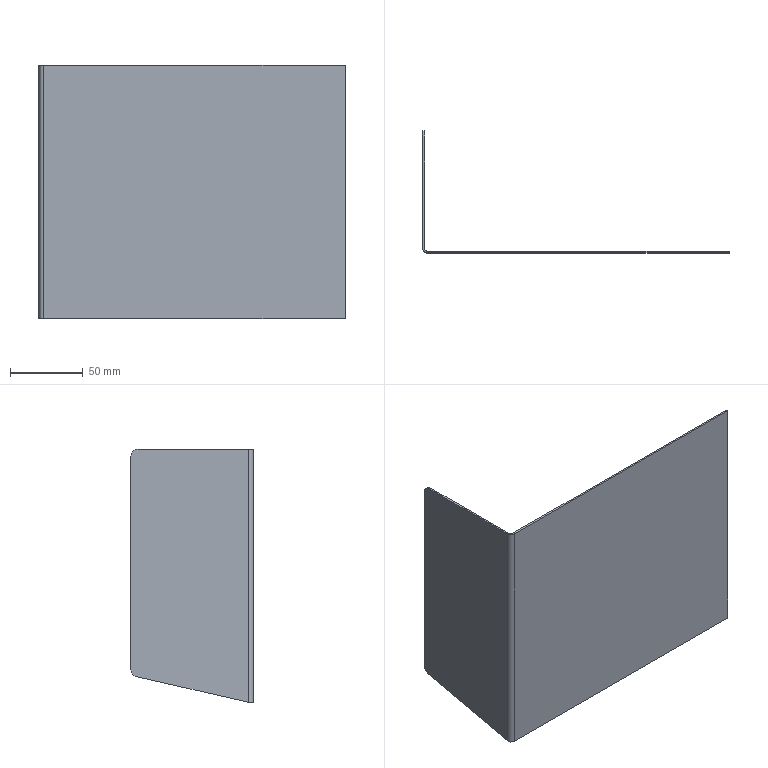Part | SolidWorks | features Fillet 1, FlatPattern 1, ICE 1, SMBaseFlange 1, SheetMetal 1 | 1 solid | 17 faces | box 211.2 x 84.2 x 175 mm | volume 60591 mm3 | plane 12 | cylinder 4 | spline 1 | commonest cylinder face diameters 10 x2 4 x1 6.4 x1
STEP:
#1=CARTESIAN_POINT('',(0.702,-83.,0.));
#2=VERTEX_POINT('',#1);
#3=CARTESIAN_POINT('',(3.2,-84.2,0.));
#4=VERTEX_POINT('',#3);
#5=CARTESIAN_POINT('',(3.2,-81.,0.));
#6=DIRECTION('',(0.,0.,1.));
#7=DIRECTION('',(-1.,0.,0.));
#8=AXIS2_PLACEMENT_3D('',#5,#6,#7);
#9=CIRCLE('',#8,3.2);
#10=EDGE_CURVE('',#2,#4,#9,.T.);
#11=ORIENTED_EDGE('',*,*,#10,.F.);
#12=CARTESIAN_POINT('',(1.639,-82.25,0.));
#13=VERTEX_POINT('',#12);
#14=CARTESIAN_POINT('',(0.702,-83.,0.));
#15=DIRECTION('',(0.7806,0.625,0.));
#16=VECTOR('',#15,1000.);
#17=LINE('',#14,#16);
#18=EDGE_CURVE('',#2,#13,#17,.T.);
#19=ORIENTED_EDGE('',*,*,#18,.T.);
#20=CARTESIAN_POINT('',(3.2,-83.,0.));
#21=VERTEX_POINT('',#20);
#22=CARTESIAN_POINT('',(3.2,-81.,0.));
#23=DIRECTION('',(0.,0.,1.));
#24=DIRECTION('',(1.,0.,0.));
#25=AXIS2_PLACEMENT_3D('',#22,#23,#24);
#26=CIRCLE('',#25,2.);
#27=EDGE_CURVE('',#13,#21,#26,.T.);
#28=ORIENTED_EDGE('',*,*,#27,.T.);
#29=CARTESIAN_POINT('',(3.2,-84.2,0.));
#30=DIRECTION('',(0.,1.,0.));
#31=VECTOR('',#30,1000.);
#32=LINE('',#29,#31);
#33=EDGE_CURVE('',#4,#21,#32,.T.);
#34=ORIENTED_EDGE('',*,*,#33,.F.);
#35=EDGE_LOOP('',(#11,#19,#28,#34));
#36=FACE_OUTER_BOUND('',#35,.T.);
#37=CARTESIAN_POINT('',(3.2,-84.2,0.));
#38=DIRECTION('',(0.,0.,-1.));
#39=DIRECTION('',(-1.,0.,0.));
#40=AXIS2_PLACEMENT_3D('',#37,#38,#39);
#41=PLANE('',#40);
#42=ADVANCED_FACE('',(#36),#41,.T.);
#43=ORIENTED_EDGE('',*,*,#27,.F.);
#44=CARTESIAN_POINT('',(1.2,-81.,0.4578));
#45=VERTEX_POINT('',#44);
#46=CARTESIAN_POINT('',(1.639,-82.25,0.));
#47=CARTESIAN_POINT('',(1.352,-81.892,0.1312));
#48=CARTESIAN_POINT('',(1.2,-81.459,0.2898));
#49=CARTESIAN_POINT('',(1.2,-81.,0.4578));
#50=(BOUNDED_CURVE()B_SPLINE_CURVE(3,(#46,#47,#48,#49),.UNSPECIFIED.,.F.,.T.)B_SPLINE_CURVE_WITH_KNOTS((4,4),(0.8957,1.571),.UNSPECIFIED.)CURVE()GEOMETRIC_REPRESENTATION_ITEM()RATIONAL_B_SPLINE_CURVE((1.,0.9624,0.9624,1.))REPRESENTATION_ITEM(''));
#51=EDGE_CURVE('',#13,#45,#50,.T.);
#52=ORIENTED_EDGE('',*,*,#51,.T.);
#53=CARTESIAN_POINT('',(1.2,-81.,175.));
#54=VERTEX_POINT('',#53);
#55=CARTESIAN_POINT('',(1.2,-81.,175.));
#56=DIRECTION('',(0.,0.,-1.));
#57=VECTOR('',#56,1000.);
#58=LINE('',#55,#57);
#59=EDGE_CURVE('',#54,#45,#58,.T.);
#60=ORIENTED_EDGE('',*,*,#59,.F.);
#61=CARTESIAN_POINT('',(3.2,-83.,175.));
#62=VERTEX_POINT('',#61);
#63=CARTESIAN_POINT('',(3.2,-81.,175.));
#64=DIRECTION('',(0.,0.,1.));
#65=DIRECTION('',(1.,0.,0.));
#66=AXIS2_PLACEMENT_3D('',#63,#64,#65);
#67=CIRCLE('',#66,2.);
#68=EDGE_CURVE('',#54,#62,#67,.T.);
#69=ORIENTED_EDGE('',*,*,#68,.T.);
#70=CARTESIAN_POINT('',(3.2,-83.,175.));
#71=DIRECTION('',(0.,0.,-1.));
#72=VECTOR('',#71,1000.);
#73=LINE('',#70,#72);
#74=EDGE_CURVE('',#62,#21,#73,.T.);
#75=ORIENTED_EDGE('',*,*,#74,.T.);
#76=EDGE_LOOP('',(#43,#52,#60,#69,#75));
#77=FACE_OUTER_BOUND('',#76,.T.);
#78=CARTESIAN_POINT('',(3.2,-81.,175.));
#79=DIRECTION('',(0.,0.,-1.));
#80=DIRECTION('',(-1.,0.,0.));
#81=AXIS2_PLACEMENT_3D('',#78,#79,#80);
#82=CYLINDRICAL_SURFACE('',#81,2.);
#83=ADVANCED_FACE('',(#77),#82,.F.);
#84=CARTESIAN_POINT('',(1.2,-3.884,18.111));
#85=VERTEX_POINT('',#84);
#86=CARTESIAN_POINT('',(1.2,0.,19.));
#87=DIRECTION('',(0.,0.9748,0.2231));
#88=VECTOR('',#87,1000.);
#89=LINE('',#86,#88);
#90=EDGE_CURVE('',#45,#85,#89,.T.);
#91=ORIENTED_EDGE('',*,*,#90,.T.);
#92=CARTESIAN_POINT('',(1.2,0.,22.985));
#93=VERTEX_POINT('',#92);
#94=CARTESIAN_POINT('',(1.2,-5.,22.985));
#95=DIRECTION('',(1.,0.,0.));
#96=DIRECTION('',(0.,1.,0.));
#97=AXIS2_PLACEMENT_3D('',#94,#95,#96);
#98=CIRCLE('',#97,5.);
#99=EDGE_CURVE('',#85,#93,#98,.T.);
#100=ORIENTED_EDGE('',*,*,#99,.T.);
#101=CARTESIAN_POINT('',(1.2,0.,170.));
#102=VERTEX_POINT('',#101);
#103=CARTESIAN_POINT('',(1.2,0.,175.));
#104=DIRECTION('',(0.,0.,-1.));
#105=VECTOR('',#104,1000.);
#106=LINE('',#103,#105);
#107=EDGE_CURVE('',#102,#93,#106,.T.);
#108=ORIENTED_EDGE('',*,*,#107,.F.);
#109=CARTESIAN_POINT('',(1.2,-5.,175.));
#110=VERTEX_POINT('',#109);
#111=CARTESIAN_POINT('',(1.2,-5.,170.));
#112=DIRECTION('',(1.,0.,0.));
#113=DIRECTION('',(0.,1.,0.));
#114=AXIS2_PLACEMENT_3D('',#111,#112,#113);
#115=CIRCLE('',#114,5.);
#116=EDGE_CURVE('',#102,#110,#115,.T.);
#117=ORIENTED_EDGE('',*,*,#116,.T.);
#118=CARTESIAN_POINT('',(1.2,0.,175.));
#119=DIRECTION('',(0.,-1.,0.));
#120=VECTOR('',#119,1000.);
#121=LINE('',#118,#120);
#122=EDGE_CURVE('',#110,#54,#121,.T.);
#123=ORIENTED_EDGE('',*,*,#122,.T.);
#124=ORIENTED_EDGE('',*,*,#59,.T.);
#125=EDGE_LOOP('',(#91,#100,#108,#117,#123,#124));
#126=FACE_OUTER_BOUND('',#125,.T.);
#127=CARTESIAN_POINT('',(1.2,0.,175.));
#128=DIRECTION('',(1.,0.,0.));
#129=DIRECTION('',(0.,1.,0.));
#130=AXIS2_PLACEMENT_3D('',#127,#128,#129);
#131=PLANE('',#130);
#132=ADVANCED_FACE('',(#126),#131,.T.);
#133=ORIENTED_EDGE('',*,*,#107,.T.);
#134=CARTESIAN_POINT('',(0.,0.,22.985));
#135=VERTEX_POINT('',#134);
#136=CARTESIAN_POINT('',(0.,0.,22.985));
#137=DIRECTION('',(-1.,0.,0.));
#138=VECTOR('',#137,1000.);
#139=LINE('',#136,#138);
#140=EDGE_CURVE('',#93,#135,#139,.T.);
#141=ORIENTED_EDGE('',*,*,#140,.T.);
#142=CARTESIAN_POINT('',(0.,0.,170.));
#143=VERTEX_POINT('',#142);
#144=CARTESIAN_POINT('',(0.,0.,175.));
#145=DIRECTION('',(0.,0.,-1.));
#146=VECTOR('',#145,1000.);
#147=LINE('',#144,#146);
#148=EDGE_CURVE('',#143,#135,#147,.T.);
#149=ORIENTED_EDGE('',*,*,#148,.F.);
#150=CARTESIAN_POINT('',(0.,0.,170.));
#151=DIRECTION('',(1.,0.,0.));
#152=VECTOR('',#151,1000.);
#153=LINE('',#150,#152);
#154=EDGE_CURVE('',#143,#102,#153,.T.);
#155=ORIENTED_EDGE('',*,*,#154,.T.);
#156=EDGE_LOOP('',(#133,#141,#149,#155));
#157=FACE_OUTER_BOUND('',#156,.T.);
#158=CARTESIAN_POINT('',(0.,0.,175.));
#159=DIRECTION('',(0.,1.,0.));
#160=DIRECTION('',(-1.,0.,0.));
#161=AXIS2_PLACEMENT_3D('',#158,#159,#160);
#162=PLANE('',#161);
#163=ADVANCED_FACE('',(#157),#162,.T.);
#164=ORIENTED_EDGE('',*,*,#148,.T.);
#165=CARTESIAN_POINT('',(0.,-3.884,18.111));
#166=VERTEX_POINT('',#165);
#167=CARTESIAN_POINT('',(0.,-5.,22.985));
#168=DIRECTION('',(-1.,0.,0.));
#169=DIRECTION('',(0.,1.,0.));
#170=AXIS2_PLACEMENT_3D('',#167,#168,#169);
#171=CIRCLE('',#170,5.);
#172=EDGE_CURVE('',#135,#166,#171,.T.);
#173=ORIENTED_EDGE('',*,*,#172,.T.);
#174=CARTESIAN_POINT('',(0.,-81.,0.4578));
#175=VERTEX_POINT('',#174);
#176=CARTESIAN_POINT('',(0.,0.,19.));
#177=DIRECTION('',(0.,0.9748,0.2231));
#178=VECTOR('',#177,1000.);
#179=LINE('',#176,#178);
#180=EDGE_CURVE('',#175,#166,#179,.T.);
#181=ORIENTED_EDGE('',*,*,#180,.F.);
#182=CARTESIAN_POINT('',(0.,-81.,175.));
#183=VERTEX_POINT('',#182);
#184=CARTESIAN_POINT('',(0.,-81.,175.));
#185=DIRECTION('',(0.,0.,-1.));
#186=VECTOR('',#185,1000.);
#187=LINE('',#184,#186);
#188=EDGE_CURVE('',#183,#175,#187,.T.);
#189=ORIENTED_EDGE('',*,*,#188,.F.);
#190=CARTESIAN_POINT('',(0.,-5.,175.));
#191=VERTEX_POINT('',#190);
#192=CARTESIAN_POINT('',(0.,0.,175.));
#193=DIRECTION('',(0.,-1.,0.));
#194=VECTOR('',#193,1000.);
#195=LINE('',#192,#194);
#196=EDGE_CURVE('',#191,#183,#195,.T.);
#197=ORIENTED_EDGE('',*,*,#196,.F.);
#198=CARTESIAN_POINT('',(0.,-5.,170.));
#199=DIRECTION('',(-1.,0.,0.));
#200=DIRECTION('',(0.,1.,0.));
#201=AXIS2_PLACEMENT_3D('',#198,#199,#200);
#202=CIRCLE('',#201,5.);
#203=EDGE_CURVE('',#191,#143,#202,.T.);
#204=ORIENTED_EDGE('',*,*,#203,.T.);
#205=EDGE_LOOP('',(#164,#173,#181,#189,#197,#204));
#206=FACE_OUTER_BOUND('',#205,.T.);
#207=CARTESIAN_POINT('',(0.,0.,175.));
#208=DIRECTION('',(1.,0.,0.));
#209=DIRECTION('',(0.,1.,0.));
#210=AXIS2_PLACEMENT_3D('',#207,#208,#209);
#211=PLANE('',#210);
#212=ADVANCED_FACE('',(#206),#211,.F.);
#213=CARTESIAN_POINT('',(0.702,-83.,0.));
#214=CARTESIAN_POINT('',(0.2431,-82.427,0.1312));
#215=CARTESIAN_POINT('',(0.,-81.734,0.2898));
#216=CARTESIAN_POINT('',(0.,-81.,0.4578));
#217=(BOUNDED_CURVE()B_SPLINE_CURVE(3,(#213,#214,#215,#216),.UNSPECIFIED.,.F.,.T.)B_SPLINE_CURVE_WITH_KNOTS((4,4),(0.8957,1.571),.UNSPECIFIED.)CURVE()GEOMETRIC_REPRESENTATION_ITEM()RATIONAL_B_SPLINE_CURVE((1.,0.9624,0.9624,1.))REPRESENTATION_ITEM(''));
#218=EDGE_CURVE('',#2,#175,#217,.T.);
#219=ORIENTED_EDGE('',*,*,#218,.F.);
#220=ORIENTED_EDGE('',*,*,#10,.T.);
#221=CARTESIAN_POINT('',(3.2,-84.2,175.));
#222=VERTEX_POINT('',#221);
#223=CARTESIAN_POINT('',(3.2,-84.2,175.));
#224=DIRECTION('',(0.,0.,-1.));
#225=VECTOR('',#224,1000.);
#226=LINE('',#223,#225);
#227=EDGE_CURVE('',#222,#4,#226,.T.);
#228=ORIENTED_EDGE('',*,*,#227,.F.);
#229=CARTESIAN_POINT('',(3.2,-81.,175.));
#230=DIRECTION('',(0.,0.,1.));
#231=DIRECTION('',(-1.,0.,0.));
#232=AXIS2_PLACEMENT_3D('',#229,#230,#231);
#233=CIRCLE('',#232,3.2);
#234=EDGE_CURVE('',#183,#222,#233,.T.);
#235=ORIENTED_EDGE('',*,*,#234,.F.);
#236=ORIENTED_EDGE('',*,*,#188,.T.);
#237=EDGE_LOOP('',(#219,#220,#228,#235,#236));
#238=FACE_OUTER_BOUND('',#237,.T.);
#239=CARTESIAN_POINT('',(3.2,-81.,175.));
#240=DIRECTION('',(0.,0.,-1.));
#241=DIRECTION('',(-1.,0.,0.));
#242=AXIS2_PLACEMENT_3D('',#239,#240,#241);
#243=CYLINDRICAL_SURFACE('',#242,3.2);
#244=ADVANCED_FACE('',(#238),#243,.T.);
#245=CARTESIAN_POINT('',(0.,-81.,175.));
#246=DIRECTION('',(1.,0.,0.));
#247=VECTOR('',#246,1000.);
#248=LINE('',#245,#247);
#249=EDGE_CURVE('',#183,#54,#248,.T.);
#250=ORIENTED_EDGE('',*,*,#249,.F.);
#251=ORIENTED_EDGE('',*,*,#234,.T.);
#252=CARTESIAN_POINT('',(3.2,-83.,175.));
#253=DIRECTION('',(0.,-1.,0.));
#254=VECTOR('',#253,1000.);
#255=LINE('',#252,#254);
#256=EDGE_CURVE('',#62,#222,#255,.T.);
#257=ORIENTED_EDGE('',*,*,#256,.F.);
#258=ORIENTED_EDGE('',*,*,#68,.F.);
#259=EDGE_LOOP('',(#250,#251,#257,#258));
#260=FACE_OUTER_BOUND('',#259,.T.);
#261=CARTESIAN_POINT('',(0.,-81.,175.));
#262=DIRECTION('',(0.,0.,1.));
#263=DIRECTION('',(1.,0.,0.));
#264=AXIS2_PLACEMENT_3D('',#261,#262,#263);
#265=PLANE('',#264);
#266=ADVANCED_FACE('',(#260),#265,.T.);
#267=ORIENTED_EDGE('',*,*,#122,.F.);
#268=CARTESIAN_POINT('',(3.2,-5.,175.));
#269=DIRECTION('',(-1.,0.,0.));
#270=VECTOR('',#269,1000.);
#271=LINE('',#268,#270);
#272=EDGE_CURVE('',#110,#191,#271,.T.);
#273=ORIENTED_EDGE('',*,*,#272,.T.);
#274=ORIENTED_EDGE('',*,*,#196,.T.);
#275=ORIENTED_EDGE('',*,*,#249,.T.);
#276=EDGE_LOOP('',(#267,#273,#274,#275));
#277=FACE_OUTER_BOUND('',#276,.T.);
#278=CARTESIAN_POINT('',(3.2,-83.,175.));
#279=DIRECTION('',(0.,0.,1.));
#280=DIRECTION('',(1.,0.,0.));
#281=AXIS2_PLACEMENT_3D('',#278,#279,#280);
#282=PLANE('',#281);
#283=ADVANCED_FACE('',(#277),#282,.T.);
#284=CARTESIAN_POINT('',(211.2,-84.2,0.));
#285=VERTEX_POINT('',#284);
#286=CARTESIAN_POINT('',(0.,-84.2,0.));
#287=DIRECTION('',(1.,0.,0.));
#288=VECTOR('',#287,1000.);
#289=LINE('',#286,#288);
#290=EDGE_CURVE('',#4,#285,#289,.T.);
#291=ORIENTED_EDGE('',*,*,#290,.F.);
#292=ORIENTED_EDGE('',*,*,#33,.T.);
#293=CARTESIAN_POINT('',(211.2,-83.,0.));
#294=VERTEX_POINT('',#293);
#295=CARTESIAN_POINT('',(0.,-83.,0.));
#296=DIRECTION('',(1.,0.,0.));
#297=VECTOR('',#296,1000.);
#298=LINE('',#295,#297);
#299=EDGE_CURVE('',#21,#294,#298,.T.);
#300=ORIENTED_EDGE('',*,*,#299,.T.);
#301=CARTESIAN_POINT('',(211.2,-83.,0.));
#302=DIRECTION('',(0.,-1.,0.));
#303=VECTOR('',#302,1000.);
#304=LINE('',#301,#303);
#305=EDGE_CURVE('',#294,#285,#304,.T.);
#306=ORIENTED_EDGE('',*,*,#305,.T.);
#307=EDGE_LOOP('',(#291,#292,#300,#306));
#308=FACE_OUTER_BOUND('',#307,.T.);
#309=CARTESIAN_POINT('',(1.2,-81.,0.));
#310=DIRECTION('',(0.,0.,-1.));
#311=DIRECTION('',(-1.,0.,0.));
#312=AXIS2_PLACEMENT_3D('',#309,#310,#311);
#313=PLANE('',#312);
#314=ADVANCED_FACE('',(#308),#313,.T.);
#315=ORIENTED_EDGE('',*,*,#290,.T.);
#316=CARTESIAN_POINT('',(211.2,-84.2,175.));
#317=VERTEX_POINT('',#316);
#318=CARTESIAN_POINT('',(211.2,-84.2,175.));
#319=DIRECTION('',(0.,0.,-1.));
#320=VECTOR('',#319,1000.);
#321=LINE('',#318,#320);
#322=EDGE_CURVE('',#317,#285,#321,.T.);
#323=ORIENTED_EDGE('',*,*,#322,.F.);
#324=CARTESIAN_POINT('',(0.,-84.2,175.));
#325=DIRECTION('',(1.,0.,0.));
#326=VECTOR('',#325,1000.);
#327=LINE('',#324,#326);
#328=EDGE_CURVE('',#222,#317,#327,.T.);
#329=ORIENTED_EDGE('',*,*,#328,.F.);
#330=ORIENTED_EDGE('',*,*,#227,.T.);
#331=EDGE_LOOP('',(#315,#323,#329,#330));
#332=FACE_OUTER_BOUND('',#331,.T.);
#333=CARTESIAN_POINT('',(0.,-84.2,175.));
#334=DIRECTION('',(0.,1.,0.));
#335=DIRECTION('',(0.,0.,1.));
#336=AXIS2_PLACEMENT_3D('',#333,#334,#335);
#337=PLANE('',#336);
#338=ADVANCED_FACE('',(#332),#337,.F.);
#339=ORIENTED_EDGE('',*,*,#305,.F.);
#340=CARTESIAN_POINT('',(211.2,-83.,175.));
#341=VERTEX_POINT('',#340);
#342=CARTESIAN_POINT('',(211.2,-83.,175.));
#343=DIRECTION('',(0.,0.,-1.));
#344=VECTOR('',#343,1000.);
#345=LINE('',#342,#344);
#346=EDGE_CURVE('',#341,#294,#345,.T.);
#347=ORIENTED_EDGE('',*,*,#346,.F.);
#348=CARTESIAN_POINT('',(211.2,-83.,175.));
#349=DIRECTION('',(0.,-1.,0.));
#350=VECTOR('',#349,1000.);
#351=LINE('',#348,#350);
#352=EDGE_CURVE('',#341,#317,#351,.T.);
#353=ORIENTED_EDGE('',*,*,#352,.T.);
#354=ORIENTED_EDGE('',*,*,#322,.T.);
#355=EDGE_LOOP('',(#339,#347,#353,#354));
#356=FACE_OUTER_BOUND('',#355,.T.);
#357=CARTESIAN_POINT('',(211.2,-83.,175.));
#358=DIRECTION('',(1.,0.,0.));
#359=DIRECTION('',(0.,0.,-1.));
#360=AXIS2_PLACEMENT_3D('',#357,#358,#359);
#361=PLANE('',#360);
#362=ADVANCED_FACE('',(#356),#361,.T.);
#363=ORIENTED_EDGE('',*,*,#299,.F.);
#364=ORIENTED_EDGE('',*,*,#74,.F.);
#365=CARTESIAN_POINT('',(0.,-83.,175.));
#366=DIRECTION('',(1.,0.,0.));
#367=VECTOR('',#366,1000.);
#368=LINE('',#365,#367);
#369=EDGE_CURVE('',#62,#341,#368,.T.);
#370=ORIENTED_EDGE('',*,*,#369,.T.);
#371=ORIENTED_EDGE('',*,*,#346,.T.);
#372=EDGE_LOOP('',(#363,#364,#370,#371));
#373=FACE_OUTER_BOUND('',#372,.T.);
#374=CARTESIAN_POINT('',(0.,-83.,175.));
#375=DIRECTION('',(0.,1.,0.));
#376=DIRECTION('',(0.,0.,1.));
#377=AXIS2_PLACEMENT_3D('',#374,#375,#376);
#378=PLANE('',#377);
#379=ADVANCED_FACE('',(#373),#378,.T.);
#380=ORIENTED_EDGE('',*,*,#328,.T.);
#381=ORIENTED_EDGE('',*,*,#352,.F.);
#382=ORIENTED_EDGE('',*,*,#369,.F.);
#383=ORIENTED_EDGE('',*,*,#256,.T.);
#384=EDGE_LOOP('',(#380,#381,#382,#383));
#385=FACE_OUTER_BOUND('',#384,.T.);
#386=CARTESIAN_POINT('',(3.2,-81.,175.));
#387=DIRECTION('',(0.,0.,1.));
#388=DIRECTION('',(1.,0.,0.));
#389=AXIS2_PLACEMENT_3D('',#386,#387,#388);
#390=PLANE('',#389);
#391=ADVANCED_FACE('',(#385),#390,.T.);
#392=ORIENTED_EDGE('',*,*,#180,.T.);
#393=CARTESIAN_POINT('',(0.,-3.884,18.111));
#394=DIRECTION('',(1.,0.,0.));
#395=VECTOR('',#394,1000.);
#396=LINE('',#393,#395);
#397=EDGE_CURVE('',#166,#85,#396,.T.);
#398=ORIENTED_EDGE('',*,*,#397,.T.);
#399=ORIENTED_EDGE('',*,*,#90,.F.);
#400=CARTESIAN_POINT('',(0.,-81.,0.4578));
#401=DIRECTION('',(1.,0.,0.));
#402=VECTOR('',#401,1000.);
#403=LINE('',#400,#402);
#404=EDGE_CURVE('',#175,#45,#403,.T.);
#405=ORIENTED_EDGE('',*,*,#404,.F.);
#406=EDGE_LOOP('',(#392,#398,#399,#405));
#407=FACE_OUTER_BOUND('',#406,.T.);
#408=CARTESIAN_POINT('',(0.,0.,19.));
#409=DIRECTION('',(0.,0.2231,-0.9748));
#410=DIRECTION('',(0.,0.9748,0.2231));
#411=AXIS2_PLACEMENT_3D('',#408,#409,#410);
#412=PLANE('',#411);
#413=ADVANCED_FACE('',(#407),#412,.T.);
#414=ORIENTED_EDGE('',*,*,#18,.F.);
#415=ORIENTED_EDGE('',*,*,#218,.T.);
#416=ORIENTED_EDGE('',*,*,#404,.T.);
#417=ORIENTED_EDGE('',*,*,#51,.F.);
#418=EDGE_LOOP('',(#414,#415,#416,#417));
#419=FACE_OUTER_BOUND('',#418,.T.);
#420=CARTESIAN_POINT('',(3.2,-84.2,-0.2747));
#421=CARTESIAN_POINT('',(3.2,-83.8,-0.2747));
#422=CARTESIAN_POINT('',(3.2,-83.4,-0.2747));
#423=CARTESIAN_POINT('',(3.2,-83.,-0.2747));
#424=CARTESIAN_POINT('',(-3.2,-84.2,-0.2747));
#425=CARTESIAN_POINT('',(-2.4,-83.8,-0.2747));
#426=CARTESIAN_POINT('',(-1.6,-83.4,-0.2747));
#427=CARTESIAN_POINT('',(-0.8,-83.,-0.2747));
#428=CARTESIAN_POINT('',(-3.2,-77.8,1.19));
#429=CARTESIAN_POINT('',(-2.4,-78.2,1.19));
#430=CARTESIAN_POINT('',(-1.6,-78.6,1.19));
#431=CARTESIAN_POINT('',(-0.8,-79.,1.19));
#432=CARTESIAN_POINT('',(3.2,-77.8,1.19));
#433=CARTESIAN_POINT('',(3.2,-78.2,1.19));
#434=CARTESIAN_POINT('',(3.2,-78.6,1.19));
#435=CARTESIAN_POINT('',(3.2,-79.,1.19));
#436=CARTESIAN_POINT('',(9.6,-77.8,1.19));
#437=CARTESIAN_POINT('',(8.8,-78.2,1.19));
#438=CARTESIAN_POINT('',(8.,-78.6,1.19));
#439=CARTESIAN_POINT('',(7.2,-79.,1.19));
#440=CARTESIAN_POINT('',(9.6,-84.2,-0.2747));
#441=CARTESIAN_POINT('',(8.8,-83.8,-0.2747));
#442=CARTESIAN_POINT('',(8.,-83.4,-0.2747));
#443=CARTESIAN_POINT('',(7.2,-83.,-0.2747));
#444=CARTESIAN_POINT('',(3.2,-84.2,-0.2747));
#445=CARTESIAN_POINT('',(3.2,-83.8,-0.2747));
#446=CARTESIAN_POINT('',(3.2,-83.4,-0.2747));
#447=CARTESIAN_POINT('',(3.2,-83.,-0.2747));
#448=(BOUNDED_SURFACE()B_SPLINE_SURFACE(3,3,((#420,#421,#422,#423),(#424,#425,#426,#427),(#428,#429,#430,#431),(#432,#433,#434,#435),(#436,#437,#438,#439),(#440,#441,#442,#443),(#444,#445,#446,#447)),.UNSPECIFIED.,.T.,.F.,.T.)B_SPLINE_SURFACE_WITH_KNOTS((4,3,4),(4,4),(0.,0.5,1.),(0.,1.),.UNSPECIFIED.)GEOMETRIC_REPRESENTATION_ITEM()RATIONAL_B_SPLINE_SURFACE(((1.,1.,1.,1.),(0.3333,0.3333,0.3333,0.3333),(0.3333,0.3333,0.3333,0.3333),(1.,1.,1.,1.),(0.3333,0.3333,0.3333,0.3333),(0.3333,0.3333,0.3333,0.3333),(1.,1.,1.,1.)))REPRESENTATION_ITEM('')SURFACE());
#449=ADVANCED_FACE('',(#419),#448,.T.);
#450=ORIENTED_EDGE('',*,*,#172,.F.);
#451=ORIENTED_EDGE('',*,*,#140,.F.);
#452=ORIENTED_EDGE('',*,*,#99,.F.);
#453=ORIENTED_EDGE('',*,*,#397,.F.);
#454=EDGE_LOOP('',(#450,#451,#452,#453));
#455=FACE_OUTER_BOUND('',#454,.T.);
#456=CARTESIAN_POINT('',(0.,-5.,22.985));
#457=DIRECTION('',(1.,0.,0.));
#458=DIRECTION('',(0.,1.,0.));
#459=AXIS2_PLACEMENT_3D('',#456,#457,#458);
#460=CYLINDRICAL_SURFACE('',#459,5.);
#461=ADVANCED_FACE('',(#455),#460,.T.);
#462=ORIENTED_EDGE('',*,*,#203,.F.);
#463=ORIENTED_EDGE('',*,*,#272,.F.);
#464=ORIENTED_EDGE('',*,*,#116,.F.);
#465=ORIENTED_EDGE('',*,*,#154,.F.);
#466=EDGE_LOOP('',(#462,#463,#464,#465));
#467=FACE_OUTER_BOUND('',#466,.T.);
#468=CARTESIAN_POINT('',(0.,-5.,170.));
#469=DIRECTION('',(1.,0.,0.));
#470=DIRECTION('',(0.,1.,0.));
#471=AXIS2_PLACEMENT_3D('',#468,#469,#470);
#472=CYLINDRICAL_SURFACE('',#471,5.);
#473=ADVANCED_FACE('',(#467),#472,.T.);
#474=CLOSED_SHELL('',(#42,#83,#132,#163,#212,#244,#266,#283,#314,#338,#362,#379,#391,#413,#449,#461,#473));
#475=MANIFOLD_SOLID_BREP('',#474);
#476=CARTESIAN_POINT('',(0.,0.,0.));
#477=DIRECTION('',(0.,0.,1.));
#478=DIRECTION('',(1.,0.,0.));
#479=AXIS2_PLACEMENT_3D('',#476,#477,#478);
#480=(LENGTH_UNIT()NAMED_UNIT(*)SI_UNIT(.MILLI.,.METRE.));
#481=UNCERTAINTY_MEASURE_WITH_UNIT(LENGTH_MEASURE(0.00001),#480,'','');
#482=(NAMED_UNIT(*)PLANE_ANGLE_UNIT()SI_UNIT($,.RADIAN.));
#483=(NAMED_UNIT(*)SI_UNIT($,.STERADIAN.)SOLID_ANGLE_UNIT());
#484=(GEOMETRIC_REPRESENTATION_CONTEXT(3)GLOBAL_UNCERTAINTY_ASSIGNED_CONTEXT((#481))GLOBAL_UNIT_ASSIGNED_CONTEXT((#480,#482,#483))REPRESENTATION_CONTEXT('',''));
#485=ADVANCED_BREP_SHAPE_REPRESENTATION('',(#475,#479),#484);